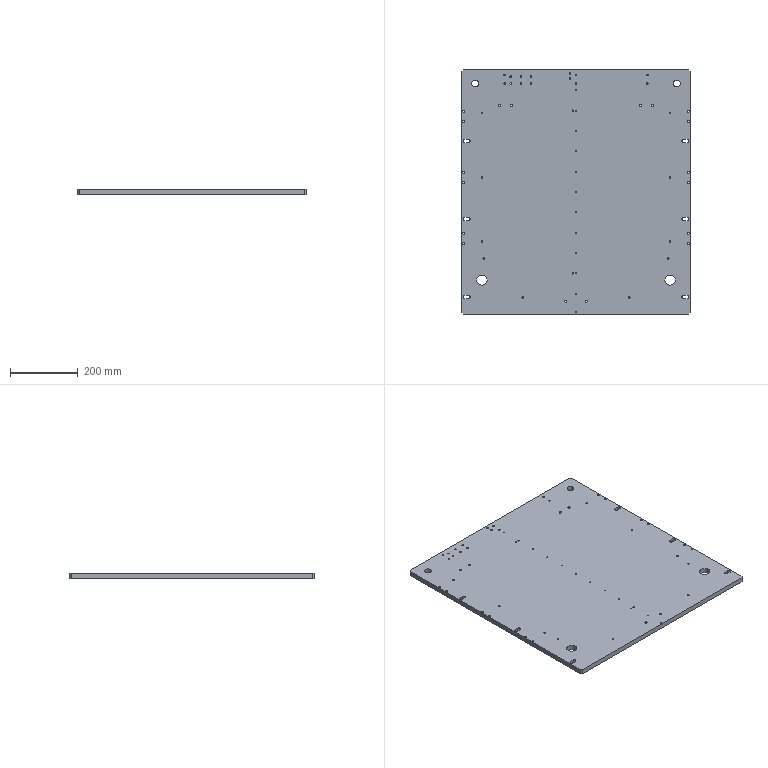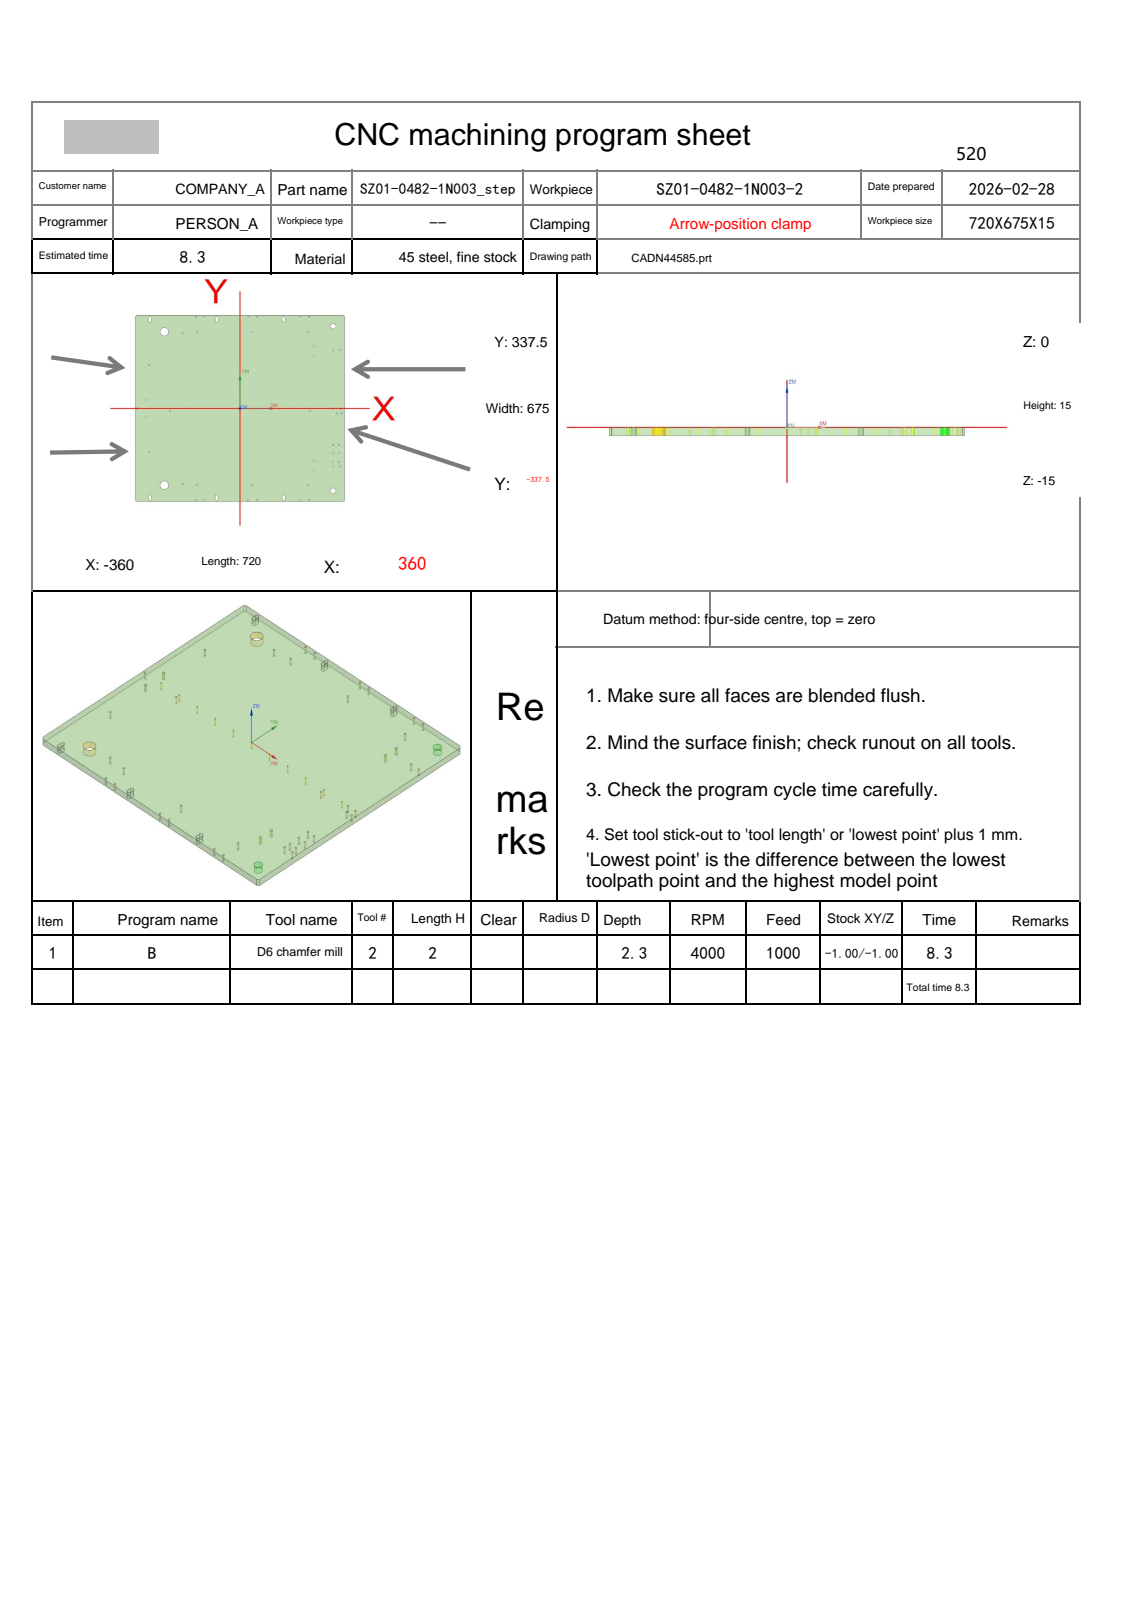NC program | NX | posted by the shop | part box 675 x 720 x 15 mm
Whole program:
%
O0001
(Machine time: 7.95 MIN)
(===Total Tool:1===)
(T2=D6 chamfer mill   D=6.   R=0.   D-  H02 Z=-2.3  )
G80 G90 G17 G49 G40
G91 G28 Z0
M01
N1 T02 M06
(D6 chamfer mill  D=6. R=0. H=02 ce=0.00 di=0.00)
G00 G90 G54 X300. Y0.0 M03 S2000
G43 H02 Z50.
M08
G98 G81 X300. Y0.0 Z-2.2 R3. F100.
X240.
X180.
X120.
X60.
X0.0
X-60.
X-120.
X-180.
X-240.
X-300.
G80
G00 Z50.
G00 G90 X240. Y-9.5 M03 S2000
Z50.
G98 G81 X240. Y-9.5 Z-2.3 R3. F100.
X-240.
G80
G00 Z50.
G00 G90 X319.306 Y-.093 M03 S4000
Z50.
Z-1.1
G01 Z-1.6 F300.
X318.5 Y-.2
G03 X320. Y-1.7 I1.5 J0.0
X321.7 Y0.0 I0.0 J1.7
X320. Y1.7 I-1.7 J0.0
X318.3 Y0.0 I0.0 J-1.7
X320. Y-1.7 I1.7 J0.0
X321.5 Y-.2 I0.0 J1.5
G01 X320.694 Y-.093
Z-1.1
G00 Z50.
X344.306
Z-1.1
G01 Z-1.6
X343.5 Y-.2
G03 X345. Y-1.7 I1.5 J0.0
X346.7 Y0.0 I0.0 J1.7
X345. Y1.7 I-1.7 J0.0
X343.3 Y0.0 I0.0 J-1.7
X345. Y-1.7 I1.7 J0.0
X346.5 Y-.2 I0.0 J1.5
G01 X345.694 Y-.093
Z-1.1
G00 Z50.
X349.306 Y-18.093
Z-1.1
G01 Z-1.6
X348.5 Y-18.2
G03 X350. Y-19.7 I1.5 J0.0
X351.7 Y-18. I0.0 J1.7
X350. Y-16.3 I-1.7 J0.0
X348.3 Y-18. I0.0 J-1.7
X350. Y-19.7 I1.7 J0.0
X351.5 Y-18.2 I0.0 J1.5
G01 X350.694 Y-18.093
Z-1.1
G00 Z50.
X333.306
Z-1.1
G01 Z-1.6
X332.5 Y-18.2
G03 X334. Y-19.7 I1.5 J0.0
X335.7 Y-18. I0.0 J1.7
X334. Y-16.3 I-1.7 J0.0
X332.3 Y-18. I0.0 J-1.7
X334. Y-19.7 I1.7 J0.0
X335.5 Y-18.2 I0.0 J1.5
G01 X334.694 Y-18.093
Z-1.1
G00 Z50.
X320.694 Y-132.407
Z-1.1
G01 Z-1.6
X321.5 Y-132.3
G03 X320. Y-130.8 I-1.5 J0.0
X318.3 Y-132.5 I0.0 J-1.7
X320. Y-134.2 I1.7 J0.0
X321.7 Y-132.5 I0.0 J1.7
X320. Y-130.8 I-1.7 J0.0
X318.5 Y-132.3 I0.0 J-1.5
G01 X319.306 Y-132.407
Z-1.1
G00 Z50.
X340.694
Z-1.1
G01 Z-1.6
X341.5 Y-132.3
G03 X340. Y-130.8 I-1.5 J0.0
X338.3 Y-132.5 I0.0 J-1.7
X340. Y-134.2 I1.7 J0.0
X341.7 Y-132.5 I0.0 J1.7
X340. Y-130.8 I-1.7 J0.0
X338.5 Y-132.3 I0.0 J-1.5
G01 X339.306 Y-132.407
Z-1.1
G00 Z50.
X340.694 Y-162.407
Z-1.1
G01 Z-1.6
X341.5 Y-162.3
G03 X340. Y-160.8 I-1.5 J0.0
X338.3 Y-162.5 I0.0 J-1.7
X340. Y-164.2 I1.7 J0.0
X341.7 Y-162.5 I0.0 J1.7
X340. Y-160.8 I-1.7 J0.0
X338.5 Y-162.3 I0.0 J-1.5
G01 X339.306 Y-162.407
Z-1.1
G00 Z50.
X320.694
Z-1.1
G01 Z-1.6
X321.5 Y-162.3
G03 X320. Y-160.8 I-1.5 J0.0
X318.3 Y-162.5 I0.0 J-1.7
X320. Y-164.2 I1.7 J0.0
X321.7 Y-162.5 I0.0 J1.7
X320. Y-160.8 I-1.7 J0.0
X318.5 Y-162.3 I0.0 J-1.5
G01 X319.306 Y-162.407
Z-1.1
G00 Z50.
X320.694 Y-192.407
Z-1.1
G01 Z-1.6
X321.5 Y-192.3
G03 X320. Y-190.8 I-1.5 J0.0
X318.3 Y-192.5 I0.0 J-1.7
X320. Y-194.2 I1.7 J0.0
X321.7 Y-192.5 I0.0 J1.7
X320. Y-190.8 I-1.7 J0.0
X318.5 Y-192.3 I0.0 J-1.5
G01 X319.306 Y-192.407
Z-1.1
G00 Z50.
X340.694
Z-1.1
G01 Z-1.6
X341.5 Y-192.3
G03 X340. Y-190.8 I-1.5 J0.0
X338.3 Y-192.5 I0.0 J-1.7
X340. Y-194.2 I1.7 J0.0
X341.7 Y-192.5 I0.0 J1.7
X340. Y-190.8 I-1.7 J0.0
X338.5 Y-192.3 I0.0 J-1.5
G01 X339.306 Y-192.407
Z-1.1
G00 Z50.
X344.306 Y-210.093
Z-1.1
G01 Z-1.6
X343.5 Y-210.2
G03 X345. Y-211.7 I1.5 J0.0
X346.7 Y-210. I0.0 J1.7
X345. Y-208.3 I-1.7 J0.0
X343.3 Y-210. I0.0 J-1.7
X345. Y-211.7 I1.7 J0.0
X346.5 Y-210.2 I0.0 J1.5
G01 X345.694 Y-210.093
Z-1.1
G00 Z50.
X319.306
Z-1.1
G01 Z-1.6
X318.5 Y-210.2
G03 X320. Y-211.7 I1.5 J0.0
X321.7 Y-210. I0.0 J1.7
X320. Y-208.3 I-1.7 J0.0
X318.3 Y-210. I0.0 J-1.7
X320. Y-211.7 I1.7 J0.0
X321.5 Y-210.2 I0.0 J1.5
G01 X320.694 Y-210.093
Z-1.1
G00 Z50.
X232.306 Y-277.093
Z-1.1
G01 Z-1.6
X231.5 Y-277.2
G03 X233. Y-278.7 I1.5 J0.0
X234.7 Y-277. I0.0 J1.7
X233. Y-275.3 I-1.7 J0.0
X231.3 Y-277. I0.0 J-1.7
X233. Y-278.7 I1.7 J0.0
X234.5 Y-277.2 I0.0 J1.5
G01 X233.694 Y-277.093
Z-1.1
G00 Z50.
X237.306 Y-331.593
Z-1.1
G01 Z-1.6
X236.5 Y-331.7
G03 X238. Y-333.2 I1.5 J0.0
X239.7 Y-331.5 I0.0 J1.7
X238. Y-329.8 I-1.7 J0.0
X236.3 Y-331.5 I0.0 J-1.7
X238. Y-333.2 I1.7 J0.0
X239.5 Y-331.7 I0.0 J1.5
G01 X238.694 Y-331.593
Z-1.1
G00 Z50.
X207.306
Z-1.1
G01 Z-1.6
X206.5 Y-331.7
G03 X208. Y-333.2 I1.5 J0.0
X209.7 Y-331.5 I0.0 J1.7
X208. Y-329.8 I-1.7 J0.0
X206.3 Y-331.5 I0.0 J-1.7
X208. Y-333.2 I1.7 J0.0
X209.5 Y-331.7 I0.0 J1.5
G01 X208.694 Y-331.593
Z-1.1
G00 Z50.
X57.306
Z-1.1
G01 Z-1.6
X56.5 Y-331.7
G03 X58. Y-333.2 I1.5 J0.0
X59.7 Y-331.5 I0.0 J1.7
X58. Y-329.8 I-1.7 J0.0
X56.3 Y-331.5 I0.0 J-1.7
X58. Y-333.2 I1.7 J0.0
X59.5 Y-331.7 I0.0 J1.5
G01 X58.694 Y-331.593
Z-1.1
G00 Z50.
X42.306 Y-277.093
Z-1.1
G01 Z-1.6
X41.5 Y-277.2
G03 X43. Y-278.7 I1.5 J0.0
X44.7 Y-277. I0.0 J1.7
X43. Y-275.3 I-1.7 J0.0
X41.3 Y-277. I0.0 J-1.7
X43. Y-278.7 I1.7 J0.0
X44.5 Y-277.2 I0.0 J1.5
G01 X43.694 Y-277.093
Z-1.1
G00 Z50.
X27.306 Y-331.593
Z-1.1
G01 Z-1.6
X26.5 Y-331.7
G03 X28. Y-333.2 I1.5 J0.0
X29.7 Y-331.5 I0.0 J1.7
X28. Y-329.8 I-1.7 J0.0
X26.3 Y-331.5 I0.0 J-1.7
X28. Y-333.2 I1.7 J0.0
X29.5 Y-331.7 I0.0 J1.5
G01 X28.694 Y-331.593
Z-1.1
G00 Z50.
X-122.694
Z-1.1
G01 Z-1.6
X-123.5 Y-331.7
G03 X-122. Y-333.2 I1.5 J0.0
X-120.3 Y-331.5 I0.0 J1.7
X-122. Y-329.8 I-1.7 J0.0
X-123.7 Y-331.5 I0.0 J-1.7
X-122. Y-333.2 I1.7 J0.0
X-120.5 Y-331.7 I0.0 J1.5
G01 X-121.306 Y-331.593
Z-1.1
G00 Z50.
X-152.694
Z-1.1
G01 Z-1.6
X-153.5 Y-331.7
G03 X-152. Y-333.2 I1.5 J0.0
X-150.3 Y-331.5 I0.0 J1.7
X-152. Y-329.8 I-1.7 J0.0
X-153.7 Y-331.5 I0.0 J-1.7
X-152. Y-333.2 I1.7 J0.0
X-150.5 Y-331.7 I0.0 J1.5
G01 X-151.306 Y-331.593
Z-1.1
G00 Z50.
X-147.694 Y-277.093
Z-1.1
G01 Z-1.6
X-148.5 Y-277.2
G03 X-147. Y-278.7 I1.5 J0.0
X-145.3 Y-277. I0.0 J1.7
X-147. Y-275.3 I-1.7 J0.0
X-148.7 Y-277. I0.0 J-1.7
X-147. Y-278.7 I1.7 J0.0
X-145.5 Y-277.2 I0.0 J1.5
G01 X-146.306 Y-277.093
Z-1.1
G00 Z50.
X-197.694 Y-272.024
Z-1.1
G01 Z-1.6
X-198.5 Y-272.132
G03 X-197. Y-273.632 I1.5 J0.0
X-195.3 Y-271.932 I0.0 J1.7
X-197. Y-270.232 I-1.7 J0.0
X-198.7 Y-271.932 I0.0 J-1.7
X-197. Y-273.632 I1.7 J0.0
X-195.5 Y-272.132 I0.0 J1.5
G01 X-196.306 Y-272.024
Z-1.1
G00 Z50.
X-312.626 Y-157.093
Z-1.1
G01 Z-1.6
X-313.432 Y-157.2
G03 X-311.932 Y-158.7 I1.5 J0.0
X-310.232 Y-157. I0.0 J1.7
X-311.932 Y-155.3 I-1.7 J0.0
X-313.632 Y-157. I0.0 J-1.7
X-311.932 Y-158.7 I1.7 J0.0
X-310.432 Y-157.2 I0.0 J1.5
G01 X-311.238 Y-157.093
Z-1.1
G00 Z50.
X-354.694 Y-.093
Z-1.1
G01 Z-1.6
X-355.5 Y-.2
G03 X-354. Y-1.7 I1.5 J0.0
X-352.3 Y0.0 I0.0 J1.7
X-354. Y1.7 I-1.7 J0.0
X-355.7 Y0.0 I0.0 J-1.7
X-354. Y-1.7 I1.7 J0.0
X-352.5 Y-.2 I0.0 J1.5
G01 X-353.306 Y-.093
Z-1.1
G00 Z50.
X-312.626 Y156.907
Z-1.1
G01 Z-1.6
X-313.432 Y156.8
G03 X-311.932 Y155.3 I1.5 J0.0
X-310.232 Y157. I0.0 J1.7
X-311.932 Y158.7 I-1.7 J0.0
X-313.632 Y157. I0.0 J-1.7
X-311.932 Y155.3 I1.7 J0.0
X-310.432 Y156.8 I0.0 J1.5
G01 X-311.238 Y156.907
Z-1.1
G00 Z50.
X-197.694 Y271.839
Z-1.1
G01 Z-1.6
X-198.5 Y271.732
G03 X-197. Y270.232 I1.5 J0.0
X-195.3 Y271.932 I0.0 J1.7
X-197. Y273.632 I-1.7 J0.0
X-198.7 Y271.932 I0.0 J-1.7
X-197. Y270.232 I1.7 J0.0
X-195.5 Y271.732 I0.0 J1.5
G01 X-196.306 Y271.839
Z-1.1
G00 Z50.
X-147.694 Y276.907
Z-1.1
G01 Z-1.6
X-148.5 Y276.8
G03 X-147. Y275.3 I1.5 J0.0
X-145.3 Y277. I0.0 J1.7
X-147. Y278.7 I-1.7 J0.0
X-148.7 Y277. I0.0 J-1.7
X-147. Y275.3 I1.7 J0.0
X-145.5 Y276.8 I0.0 J1.5
G01 X-146.306 Y276.907
Z-1.1
G00 Z50.
X-152.694 Y331.407
Z-1.1
G01 Z-1.6
X-153.5 Y331.3
G03 X-152. Y329.8 I1.5 J0.0
X-150.3 Y331.5 I0.0 J1.7
X-152. Y333.2 I-1.7 J0.0
X-153.7 Y331.5 I0.0 J-1.7
X-152. Y329.8 I1.7 J0.0
X-150.5 Y331.3 I0.0 J1.5
G01 X-151.306 Y331.407
Z-1.1
G00 Z50.
X-122.694
Z-1.1
G01 Z-1.6
X-123.5 Y331.3
G03 X-122. Y329.8 I1.5 J0.0
X-120.3 Y331.5 I0.0 J1.7
X-122. Y333.2 I-1.7 J0.0
X-123.7 Y331.5 I0.0 J-1.7
X-122. Y329.8 I1.7 J0.0
X-120.5 Y331.3 I0.0 J1.5
G01 X-121.306 Y331.407
Z-1.1
G00 Z50.
X27.306
Z-1.1
G01 Z-1.6
X26.5 Y331.3
G03 X28. Y329.8 I1.5 J0.0
X29.7 Y331.5 I0.0 J1.7
X28. Y333.2 I-1.7 J0.0
X26.3 Y331.5 I0.0 J-1.7
X28. Y329.8 I1.7 J0.0
X29.5 Y331.3 I0.0 J1.5
G01 X28.694 Y331.407
Z-1.1
G00 Z50.
X42.306 Y276.907
Z-1.1
G01 Z-1.6
X41.5 Y276.8
G03 X43. Y275.3 I1.5 J0.0
X44.7 Y277. I0.0 J1.7
X43. Y278.7 I-1.7 J0.0
X41.3 Y277. I0.0 J-1.7
X43. Y275.3 I1.7 J0.0
X44.5 Y276.8 I0.0 J1.5
G01 X43.694 Y276.907
Z-1.1
G00 Z50.
X57.306 Y331.407
Z-1.1
G01 Z-1.6
X56.5 Y331.3
G03 X58. Y329.8 I1.5 J0.0
X59.7 Y331.5 I0.0 J1.7
X58. Y333.2 I-1.7 J0.0
X56.3 Y331.5 I0.0 J-1.7
X58. Y329.8 I1.7 J0.0
X59.5 Y331.3 I0.0 J1.5
G01 X58.694 Y331.407
Z-1.1
G00 Z50.
X207.306
Z-1.1
G01 Z-1.6
X206.5 Y331.3
G03 X208. Y329.8 I1.5 J0.0
X209.7 Y331.5 I0.0 J1.7
X208. Y333.2 I-1.7 J0.0
X206.3 Y331.5 I0.0 J-1.7
X208. Y329.8 I1.7 J0.0
X209.5 Y331.3 I0.0 J1.5
G01 X208.694 Y331.407
Z-1.1
G00 Z50.
X237.306
Z-1.1
G01 Z-1.6
X236.5 Y331.3
G03 X238. Y329.8 I1.5 J0.0
X239.7 Y331.5 I0.0 J1.7
X238. Y333.2 I-1.7 J0.0
X236.3 Y331.5 I0.0 J-1.7
X238. Y329.8 I1.7 J0.0
X239.5 Y331.3 I0.0 J1.5
G01 X238.694 Y331.407
Z-1.1
G00 Z50.
X232.306 Y276.907
Z-1.1
G01 Z-1.6
X231.5 Y276.8
G03 X233. Y275.3 I1.5 J0.0
X234.7 Y277. I0.0 J1.7
X233. Y278.7 I-1.7 J0.0
X231.3 Y277. I0.0 J-1.7
X233. Y275.3 I1.7 J0.0
X234.5 Y276.8 I0.0 J1.5
G01 X233.694 Y276.907
Z-1.1
G00 Z50.
X319.306 Y209.907
Z-1.1
G01 Z-1.6
X318.5 Y209.8
G03 X320. Y208.3 I1.5 J0.0
X321.7 Y210. I0.0 J1.7
X320. Y211.7 I-1.7 J0.0
X318.3 Y210. I0.0 J-1.7
X320. Y208.3 I1.7 J0.0
X321.5 Y209.8 I0.0 J1.5
G01 X320.694 Y209.907
Z-1.1
G00 Z50.
X344.306
Z-1.1
G01 Z-1.6
X343.5 Y209.8
G03 X345. Y208.3 I1.5 J0.0
X346.7 Y210. I0.0 J1.7
X345. Y211.7 I-1.7 J0.0
X343.3 Y210. I0.0 J-1.7
X345. Y208.3 I1.7 J0.0
X346.5 Y209.8 I0.0 J1.5
G01 X345.694 Y209.907
Z-1.1
G00 Z50.
G00 G90 X-323.5 Y-30.995 M03 S4000
Z50.
Z-1.1
G01 Z-1.6 F300.
Y-31.3
G03 X-322. Y-32.8 I1.5 J0.0
X-319.2 Y-30. I0.0 J2.8
X-322. Y-27.2 I-2.8 J0.0
X-324.8 Y-30. I0.0 J-2.8
X-322. Y-32.8 I2.8 J0.0
X-320.5 Y-31.3 I0.0 J1.5
G01 Y-30.995
Z-1.1
G00 Z50.
X-323.5 Y29.005
Z-1.1
G01 Z-1.6
Y28.7
G03 X-322. Y27.2 I1.5 J0.0
X-319.2 Y30. I0.0 J2.8
X-322. Y32.8 I-2.8 J0.0
X-324.8 Y30. I0.0 J-2.8
X-322. Y27.2 I2.8 J0.0
X-320.5 Y28.7 I0.0 J1.5
G01 Y29.005
Z-1.1
G00 Z50.
X253.5 Y224.505
Z-1.1
G01 Z-1.6
Y224.2
G03 X255. Y222.7 I1.5 J0.0
X257.8 Y225.5 I0.0 J2.8
X255. Y228.3 I-2.8 J0.0
X252.2 Y225.5 I0.0 J-2.8
X255. Y222.7 I2.8 J0.0
X256.5 Y224.2 I0.0 J1.5
G01 Y224.505
Z-1.1
G00 Z50.
X253.5 Y188.505
Z-1.1
G01 Z-1.6
Y188.2
G03 X255. Y186.7 I1.5 J0.0
X257.8 Y189.5 I0.0 J2.8
X255. Y192.3 I-2.8 J0.0
X252.2 Y189.5 I0.0 J-2.8
X255. Y186.7 I2.8 J0.0
X256.5 Y188.2 I0.0 J1.5
G01 Y188.505
Z-1.1
G00 Z50.
X253.5 Y-190.495
Z-1.1
G01 Z-1.6
Y-190.8
G03 X255. Y-192.3 I1.5 J0.0
X257.8 Y-189.5 I0.0 J2.8
X255. Y-186.7 I-2.8 J0.0
X252.2 Y-189.5 I0.0 J-2.8
X255. Y-192.3 I2.8 J0.0
X256.5 Y-190.8 I0.0 J1.5
G01 Y-190.495
Z-1.1
G00 Z50.
X253.5 Y-226.495
Z-1.1
G01 Z-1.6
Y-226.8
G03 X255. Y-228.3 I1.5 J0.0
X257.8 Y-225.5 I0.0 J2.8
X255. Y-222.7 I-2.8 J0.0
X252.2 Y-225.5 I0.0 J-2.8
X255. Y-228.3 I2.8 J0.0
X256.5 Y-226.8 I0.0 J1.5
G01 Y-226.495
Z-1.1
G00 Z50.
G00 G90 X-361.275 Y332.147 M03 S3500
Z50.
Z.124
G01 Z-1.2 F1000.
G03 X-361.04 Y332.404 I-1.351 J1.475
G01 X-361.004 Y332.446
X-361. Y332.5
X-360.966 Y332.759
X-360.866 Y333.
X-360.707 Y333.207
X-355.707 Y338.207
X-355.5 Y338.366
X-355.259 Y338.466
X-355. Y338.5
X355.
X355.259 Y338.466
X355.5 Y338.366
X355.707 Y338.207
X360.707 Y333.207
X360.744 Y333.167
X360.797 Y333.155
G03 X361.14 Y333.095 I.518 J1.932
G01 Z.113
G00 Z50.
X361.275 Y-332.147
Z.124
G01 Z-1.2
G03 X361.04 Y-332.404 I1.351 J-1.475
G01 X361.004 Y-332.446
X361. Y-332.5
X360.966 Y-332.759
X360.866 Y-333.
X360.707 Y-333.207
X355.707 Y-338.207
X355.5 Y-338.366
X355.259 Y-338.466
X355. Y-338.5
X-355.
X-355.259 Y-338.466
X-355.5 Y-338.366
X-355.707 Y-338.207
X-360.707 Y-333.207
X-360.744 Y-333.167
X-360.797 Y-333.155
G03 X-361.14 Y-333.095 I-.518 J-1.932
G01 Z.113
G00 Z50.
X319.605 Y-306.29
Z.199
G01 Z-1.2
G03 X319.899 Y-306.478 I1.218 J1.587
G01 X319.946 Y-306.505
X320. Y-306.5
G03 X329. Y-297.5 I0.0 J9.
X320. Y-288.5 I-9. J0.0
X311. Y-297.5 I0.0 J-9.
X320. Y-306.5 I9. J0.0
G01 X320.054 Y-306.505
X320.101 Y-306.478
G03 X320.395 Y-306.29 I-.923 J1.774
G01 Z.199
G00 Z50.
X344.593 Y-211.315
Z.284
G01 Z-1.2
G03 X344.898 Y-211.484 I1.118 J1.658
G01 X344.946 Y-211.509
X345. Y-211.5
G03 X346.5 Y-210. I0.0 J1.5
X345. Y-208.5 I-1.5 J0.0
X343.5 Y-210. I0.0 J-1.5
X345. Y-211.5 I1.5 J0.0
G01 X345.054 Y-211.509
X345.102 Y-211.484
G03 X345.407 Y-211.315 I-.813 J1.827
G01 Z.284
G00 Z50.
X340.407 Y-191.185
Z.284
G01 Z-1.2
G03 X340.102 Y-191.016 I-1.118 J-1.658
G01 X340.054 Y-190.991
X340. Y-191.
G03 X338.5 Y-192.5 I0.0 J-1.5
X340. Y-194. I1.5 J0.0
X341.5 Y-192.5 I0.0 J1.5
X340. Y-191. I-1.5 J0.0
G01 X339.946 Y-190.991
X339.898 Y-191.016
G03 X339.593 Y-191.185 I.813 J-1.827
G01 Z.284
G00 Z50.
X340.407 Y-161.185
Z.284
G01 Z-1.2
G03 X340.102 Y-161.016 I-1.118 J-1.658
G01 X340.054 Y-160.991
X340. Y-161.
G03 X338.5 Y-162.5 I0.0 J-1.5
X340. Y-164. I1.5 J0.0
X341.5 Y-162.5 I0.0 J1.5
X340. Y-161. I-1.5 J0.0
G01 X339.946 Y-160.991
X339.898 Y-161.016
G03 X339.593 Y-161.185 I.813 J-1.827
G01 Z.284
G00 Z50.
X340.407 Y-131.185
Z.284
G01 Z-1.2
G03 X340.102 Y-131.016 I-1.118 J-1.658
G01 X340.054 Y-130.991
X340. Y-131.
G03 X338.5 Y-132.5 I0.0 J-1.5
X340. Y-134. I1.5 J0.0
X341.5 Y-132.5 I0.0 J1.5
X340. Y-131. I-1.5 J0.0
G01 X339.946 Y-130.991
X339.898 Y-131.016
G03 X339.593 Y-131.185 I.813 J-1.827
G01 Z.284
G00 Z50.
X320.407
Z.284
G01 Z-1.2
G03 X320.102 Y-131.016 I-1.118 J-1.658
G01 X320.054 Y-130.991
X320. Y-131.
G03 X318.5 Y-132.5 I0.0 J-1.5
X320. Y-134. I1.5 J0.0
X321.5 Y-132.5 I0.0 J1.5
X320. Y-131. I-1.5 J0.0
G01 X319.946 Y-130.991
X319.898 Y-131.016
G03 X319.593 Y-131.185 I.813 J-1.827
G01 Z.284
G00 Z50.
X320.407 Y-161.185
Z.284
G01 Z-1.2
G03 X320.102 Y-161.016 I-1.118 J-1.658
G01 X320.054 Y-160.991
X320. Y-161.
G03 X318.5 Y-162.5 I0.0 J-1.5
X320. Y-164. I1.5 J0.0
X321.5 Y-162.5 I0.0 J1.5
X320. Y-161. I-1.5 J0.0
G01 X319.946 Y-160.991
X319.898 Y-161.016
G03 X319.593 Y-161.185 I.813 J-1.827
G01 Z.284
G00 Z50.
X320.407 Y-191.185
Z.284
G01 Z-1.2
G03 X320.102 Y-191.016 I-1.118 J-1.658
G01 X320.054 Y-190.991
X320. Y-191.
G03 X318.5 Y-192.5 I0.0 J-1.5
X320. Y-194. I1.5 J0.0
X321.5 Y-192.5 I0.0 J1.5
X320. Y-191. I-1.5 J0.0
G01 X319.946 Y-190.991
X319.898 Y-191.016
G03 X319.593 Y-191.185 I.813 J-1.827
G01 Z.284
G00 Z50.
Y-211.315
Z.284
G01 Z-1.2
G03 X319.898 Y-211.484 I1.118 J1.658
G01 X319.946 Y-211.509
X320. Y-211.5
G03 X321.5 Y-210. I0.0 J1.5
X320. Y-208.5 I-1.5 J0.0
X318.5 Y-210. I0.0 J-1.5
X320. Y-211.5 I1.5 J0.0
G01 X320.054 Y-211.509
X320.102 Y-211.484
G03 X320.407 Y-211.315 I-.813 J1.827
G01 Z.284
G00 Z50.
X254.596 Y-191.708
Z.252
G01 Z-1.2
G03 X254.898 Y-191.882 I1.147 J1.638
G01 X254.946 Y-191.908
X255. Y-191.9
G03 X257.4 Y-189.5 I0.0 J2.4
X255. Y-187.1 I-2.4 J0.0
X252.6 Y-189.5 I0.0 J-2.4
X255. Y-191.9 I2.4 J0.0
G01 X255.054 Y-191.908
X255.102 Y-191.882
G03 X255.404 Y-191.708 I-.845 J1.813
G01 Z.252
G00 Z50.
X254.596 Y-227.708
Z.252
G01 Z-1.2
G03 X254.898 Y-227.882 I1.147 J1.638
G01 X254.946 Y-227.908
X255. Y-227.9
G03 X257.4 Y-225.5 I0.0 J2.4
X255. Y-223.1 I-2.4 J0.0
X252.6 Y-225.5 I0.0 J-2.4
X255. Y-227.9 I2.4 J0.0
G01 X255.054 Y-227.908
X255.102 Y-227.882
G03 X255.404 Y-227.708 I-.845 J1.813
G01 Z.252
G00 Z50.
X232.593 Y-278.315
Z.284
G01 Z-1.2
G03 X232.898 Y-278.484 I1.118 J1.658
G01 X232.946 Y-278.509
X233. Y-278.5
G03 X234.5 Y-277. I0.0 J1.5
X233. Y-275.5 I-1.5 J0.0
X231.5 Y-277. I0.0 J-1.5
X233. Y-278.5 I1.5 J0.0
G01 X233.054 Y-278.509
X233.102 Y-278.484
G03 X233.407 Y-278.315 I-.813 J1.827
G01 Z.284
G00 Z50.
X237.593 Y-332.815
Z.284
G01 Z-1.2
G03 X237.898 Y-332.984 I1.118 J1.658
G01 X237.946 Y-333.009
X238. Y-333.
G03 X239.5 Y-331.5 I0.0 J1.5
X238. Y-330. I-1.5 J0.0
X236.5 Y-331.5 I0.0 J-1.5
X238. Y-333. I1.5 J0.0
G01 X238.054 Y-333.009
X238.102 Y-332.984
G03 X238.407 Y-332.815 I-.813 J1.827
G01 Z.284
G00 Z50.
X207.593
Z.284
G01 Z-1.2
G03 X207.898 Y-332.984 I1.118 J1.658
G01 X207.946 Y-333.009
X208. Y-333.
G03 X209.5 Y-331.5 I0.0 J1.5
X208. Y-330. I-1.5 J0.0
X206.5 Y-331.5 I0.0 J-1.5
X208. Y-333. I1.5 J0.0
G01 X208.054 Y-333.009
X208.102 Y-332.984
G03 X208.407 Y-332.815 I-.813 J1.827
G01 Z.284
G00 Z50.
X153.773 Y-322.886
Z.172
G01 Z-1.2
G03 X153.973 Y-322.6 I-1.532 J1.286
G01 X154.003 Y-322.554
X154. Y-322.5
Y-317.5
G03 X150. Y-313.5 I-4. J0.0
X146. Y-317.5 I0.0 J-4.
G01 Y-327.5
G03 X150. Y-331.5 I4. J0.0
X154. Y-327.5 I0.0 J4.
G01 Y-322.5
X154.003 Y-322.446
X153.973 Y-322.4
G03 X153.773 Y-322.114 I-1.732 J-1.
G01 Z.172
G00 Z50.
X57.593 Y-332.815
Z.284
G01 Z-1.2
G03 X57.898 Y-332.984 I1.118 J1.658
G01 X57.946 Y-333.009
X58. Y-333.
G03 X59.5 Y-331.5 I0.0 J1.5
X58. Y-330. I-1.5 J0.0
X56.5 Y-331.5 I0.0 J-1.5
X58. Y-333. I1.5 J0.0
G01 X58.054 Y-333.009
X58.102 Y-332.984
G03 X58.407 Y-332.815 I-.813 J1.827
G01 Z.284
G00 Z50.
X27.593
Z.284
G01 Z-1.2
G03 X27.898 Y-332.984 I1.118 J1.658
G01 X27.946 Y-333.009
X28. Y-333.
G03 X29.5 Y-331.5 I0.0 J1.5
X28. Y-330. I-1.5 J0.0
X26.5 Y-331.5 I0.0 J-1.5
X28. Y-333. I1.5 J0.0
G01 X28.054 Y-333.009
X28.102 Y-332.984
G03 X28.407 Y-332.815 I-.813 J1.827
G01 Z.284
G00 Z50.
X42.593 Y-278.315
Z.284
G01 Z-1.2
G03 X42.898 Y-278.484 I1.118 J1.658
G01 X42.946 Y-278.509
X43. Y-278.5
G03 X44.5 Y-277. I0.0 J1.5
X43. Y-275.5 I-1.5 J0.0
X41.5 Y-277. I0.0 J-1.5
X43. Y-278.5 I1.5 J0.0
G01 X43.054 Y-278.509
X43.102 Y-278.484
G03 X43.407 Y-278.315 I-.813 J1.827
G01 Z.284
G00 Z50.
X-76.227 Y-322.886
Z.172
G01 Z-1.2
G03 X-76.027 Y-322.6 I-1.532 J1.286
G01 X-75.997 Y-322.554
X-76. Y-322.5
Y-317.5
G03 X-80. Y-313.5 I-4. J0.0
X-84. Y-317.5 I0.0 J-4.
G01 Y-327.5
G03 X-80. Y-331.5 I4. J0.0
X-76. Y-327.5 I0.0 J4.
G01 Y-322.5
X-75.997 Y-322.446
X-76.027 Y-322.4
G03 X-76.227 Y-322.114 I-1.732 J-1.
G01 Z.172
G00 Z50.
X-122.407 Y-332.815
Z.284
G01 Z-1.2
G03 X-122.102 Y-332.984 I1.118 J1.658
G01 X-122.054 Y-333.009
X-122. Y-333.
G03 X-120.5 Y-331.5 I0.0 J1.5
X-122. Y-330. I-1.5 J0.0
X-123.5 Y-331.5 I0.0 J-1.5
X-122. Y-333. I1.5 J0.0
G01 X-121.946 Y-333.009
X-121.898 Y-332.984
G03 X-121.593 Y-332.815 I-.813 J1.827
G01 Z.284
G00 Z50.
X-152.407
Z.284
G01 Z-1.2
G03 X-152.102 Y-332.984 I1.118 J1.658
G01 X-152.054 Y-333.009
X-152. Y-333.
G03 X-150.5 Y-331.5 I0.0 J1.5
X-152. Y-330. I-1.5 J0.0
X-153.5 Y-331.5 I0.0 J-1.5
X-152. Y-333. I1.5 J0.0
G01 X-151.946 Y-333.009
X-151.898 Y-332.984
G03 X-151.593 Y-332.815 I-.813 J1.827
G01 Z.284
G00 Z50.
X-147.407 Y-278.315
Z.284
G01 Z-1.2
G03 X-147.102 Y-278.484 I1.118 J1.658
G01 X-147.054 Y-278.509
X-147. Y-278.5
G03 X-145.5 Y-277. I0.0 J1.5
X-147. Y-275.5 I-1.5 J0.0
X-148.5 Y-277. I0.0 J-1.5
X-147. Y-278.5 I1.5 J0.0
G01 X-146.946 Y-278.509
X-146.898 Y-278.484
G03 X-146.593 Y-278.315 I-.813 J1.827
G01 Z.284
G00 Z50.
X-197.407 Y-273.247
Z.284
G01 Z-1.2
G03 X-197.102 Y-273.416 I1.118 J1.658
G01 X-197.054 Y-273.44
X-197. Y-273.432
G03 X-195.5 Y-271.932 I0.0 J1.5
X-197. Y-270.432 I-1.5 J0.0
X-198.5 Y-271.932 I0.0 J-1.5
X-197. Y-273.432 I1.5 J0.0
G01 X-196.946 Y-273.44
X-196.898 Y-273.416
G03 X-196.593 Y-273.247 I-.813 J1.827
G01 Z.284
G00 Z50.
X-260.394 Y-291.288
Z.196
G01 Z-1.2
G03 X-260.101 Y-291.477 I1.227 J1.579
G01 X-260.054 Y-291.505
X-260. Y-291.5
G03 X-246. Y-277.5 I0.0 J14.
X-260. Y-263.5 I-14. J0.0
X-274. Y-277.5 I0.0 J-14.
X-260. Y-291.5 I14. J0.0
G01 X-259.946 Y-291.505
X-259.899 Y-291.477
G03 X-259.606 Y-291.288 I-.935 J1.768
G01 Z.196
G00 Z50.
X-306.227 Y-322.886
Z.172
G01 Z-1.2
G03 X-306.027 Y-322.6 I-1.532 J1.286
G01 X-305.997 Y-322.554
X-306. Y-322.5
Y-317.5
G03 X-310. Y-313.5 I-4. J0.0
X-314. Y-317.5 I0.0 J-4.
G01 Y-327.5
G03 X-310. Y-331.5 I4. J0.0
X-306. Y-327.5 I0.0 J4.
G01 Y-322.5
X-305.997 Y-322.446
X-306.027 Y-322.4
G03 X-306.227 Y-322.114 I-1.732 J-1.
G01 Z.172
G00 Z50.
X-312.339 Y-158.315
Z.284
G01 Z-1.2
G03 X-312.034 Y-158.484 I1.118 J1.658
G01 X-311.986 Y-158.509
X-311.932 Y-158.5
G03 X-310.432 Y-157. I0.0 J1.5
X-311.932 Y-155.5 I-1.5 J0.0
X-313.432 Y-157. I0.0 J-1.5
X-311.932 Y-158.5 I1.5 J0.0
G01 X-311.878 Y-158.509
X-311.83 Y-158.484
G03 X-311.525 Y-158.315 I-.813 J1.827
G01 Z.284
G00 Z50.
X-322.404 Y-32.208
Z.252
G01 Z-1.2
G03 X-322.102 Y-32.382 I1.147 J1.638
G01 X-322.054 Y-32.408
X-322. Y-32.4
G03 X-319.6 Y-30. I0.0 J2.4
X-322. Y-27.6 I-2.4 J0.0
X-324.4 Y-30. I0.0 J-2.4
X-322. Y-32.4 I2.4 J0.0
G01 X-321.946 Y-32.408
X-321.898 Y-32.382
G03 X-321.596 Y-32.208 I-.845 J1.813
G01 Z.252
G00 Z50.
X-354.407 Y-1.315
Z.284
G01 Z-1.2
G03 X-354.102 Y-1.484 I1.118 J1.658
G01 X-354.054 Y-1.509
X-354. Y-1.5
G03 X-352.5 Y0.0 I0.0 J1.5
X-354. Y1.5 I-1.5 J0.0
X-355.5 Y0.0 I0.0 J-1.5
X-354. Y-1.5 I1.5 J0.0
G01 X-353.946 Y-1.509
X-353.898 Y-1.484
G03 X-353.593 Y-1.315 I-.813 J1.827
G01 Z.284
G00 Z50.
X-322.404 Y27.792
Z.252
G01 Z-1.2
G03 X-322.102 Y27.618 I1.147 J1.638
G01 X-322.054 Y27.592
X-322. Y27.6
G03 X-319.6 Y30. I0.0 J2.4
X-322. Y32.4 I-2.4 J0.0
X-324.4 Y30. I0.0 J-2.4
X-322. Y27.6 I2.4 J0.0
G01 X-321.946 Y27.592
X-321.898 Y27.618
G03 X-321.596 Y27.792 I-.845 J1.813
G01 Z.252
G00 Z50.
X-300.419 Y-.494
Z.405
G01 Z-1.2
G03 X-300.103 Y-.641 I1. J1.732
G01 X-300.053 Y-.662
X-300. Y-.65
G03 X-299.35 Y0.0 I0.0 J.65
X-300. Y.65 I-.65 J0.0
X-300.65 Y0.0 I0.0 J-.65
X-300. Y-.65 I.65 J0.0
G01 X-299.947 Y-.662
X-299.897 Y-.641
G03 X-299.581 Y-.494 I-.684 J1.879
G01 Z.405
G00 Z50.
X-240.412 Y-10.326
Z.33
G01 Z-1.2
G03 X-240.103 Y-10.486 I1.075 J1.687
G01 X-240.054 Y-10.51
X-240. Y-10.5
G03 X-239. Y-9.5 I0.0 J1.
X-240. Y-8.5 I-1. J0.0
X-241. Y-9.5 I0.0 J-1.
X-240. Y-10.5 I1. J0.0
G01 X-239.946 Y-10.51
X-239.897 Y-10.486
G03 X-239.588 Y-10.326 I-.765 J1.848
G01 Z.33
G00 Z2.55
X-240.419 Y-.494
Z.405
G01 Z-1.2
G03 X-240.103 Y-.641 I1. J1.732
G01 X-240.053 Y-.662
X-240. Y-.65
G03 X-239.35 Y0.0 I0.0 J.65
X-240. Y.65 I-.65 J0.0
X-240.65 Y0.0 I0.0 J-.65
X-240. Y-.65 I.65 J0.0
G01 X-239.947 Y-.662
X-239.897 Y-.641
G03 X-239.581 Y-.494 I-.684 J1.879
G01 Z.405
G00 Z50.
X-180.419
Z.405
G01 Z-1.2
G03 X-180.103 Y-.641 I1. J1.732
G01 X-180.053 Y-.662
X-180. Y-.65
G03 X-179.35 Y0.0 I0.0 J.65
X-180. Y.65 I-.65 J0.0
X-180.65 Y0.0 I0.0 J-.65
X-180. Y-.65 I.65 J0.0
G01 X-179.947 Y-.662
X-179.897 Y-.641
G03 X-179.581 Y-.494 I-.684 J1.879
G01 Z.405
G00 Z50.
X-120.419
Z.405
G01 Z-1.2
G03 X-120.103 Y-.641 I1. J1.732
G01 X-120.053 Y-.662
X-120. Y-.65
G03 X-119.35 Y0.0 I0.0 J.65
X-120. Y.65 I-.65 J0.0
X-120.65 Y0.0 I0.0 J-.65
X-120. Y-.65 I.65 J0.0
G01 X-119.947 Y-.662
X-119.897 Y-.641
G03 X-119.581 Y-.494 I-.684 J1.879
G01 Z.405
G00 Z50.
X-60.419
Z.405
G01 Z-1.2
G03 X-60.103 Y-.641 I1. J1.732
G01 X-60.053 Y-.662
X-60. Y-.65
G03 X-59.35 Y0.0 I0.0 J.65
X-60. Y.65 I-.65 J0.0
X-60.65 Y0.0 I0.0 J-.65
X-60. Y-.65 I.65 J0.0
G01 X-59.947 Y-.662
X-59.897 Y-.641
G03 X-59.581 Y-.494 I-.684 J1.879
G01 Z.405
G00 Z50.
X-.419
Z.405
G01 Z-1.2
G03 X-.103 Y-.641 I1. J1.732
G01 X-.053 Y-.662
X0.0 Y-.65
G03 X.65 Y0.0 I0.0 J.65
X0.0 Y.65 I-.65 J0.0
X-.65 Y0.0 I0.0 J-.65
X0.0 Y-.65 I.65 J0.0
G01 X.053 Y-.662
X.103 Y-.641
G03 X.419 Y-.494 I-.684 J1.879
G01 Z.405
G00 Z50.
X59.581
Z.405
G01 Z-1.2
G03 X59.897 Y-.641 I1. J1.732
G01 X59.947 Y-.662
X60. Y-.65
G03 X60.65 Y0.0 I0.0 J.65
X60. Y.65 I-.65 J0.0
X59.35 Y0.0 I0.0 J-.65
X60. Y-.65 I.65 J0.0
G01 X60.053 Y-.662
X60.103 Y-.641
G03 X60.419 Y-.494 I-.684 J1.879
G01 Z.405
G00 Z50.
X119.581
Z.405
G01 Z-1.2
G03 X119.897 Y-.641 I1. J1.732
G01 X119.947 Y-.662
X120. Y-.65
G03 X120.65 Y0.0 I0.0 J.65
X120. Y.65 I-.65 J0.0
X119.35 Y0.0 I0.0 J-.65
X120. Y-.65 I.65 J0.0
G01 X120.053 Y-.662
X120.103 Y-.641
G03 X120.419 Y-.494 I-.684 J1.879
G01 Z.405
G00 Z50.
X179.581
Z.405
G01 Z-1.2
G03 X179.897 Y-.641 I1. J1.732
G01 X179.947 Y-.662
X180. Y-.65
G03 X180.65 Y0.0 I0.0 J.65
X180. Y.65 I-.65 J0.0
X179.35 Y0.0 I0.0 J-.65
X180. Y-.65 I.65 J0.0
G01 X180.053 Y-.662
X180.103 Y-.641
G03 X180.419 Y-.494 I-.684 J1.879
G01 Z.405
G00 Z50.
X239.588 Y-10.326
Z.33
G01 Z-1.2
G03 X239.897 Y-10.486 I1.075 J1.687
G01 X239.946 Y-10.51
X240. Y-10.5
G03 X241. Y-9.5 I0.0 J1.
X240. Y-8.5 I-1. J0.0
X239. Y-9.5 I0.0 J-1.
X240. Y-10.5 I1. J0.0
G01 X240.054 Y-10.51
X240.103 Y-10.486
G03 X240.412 Y-10.326 I-.765 J1.848
G01 Z.33
G00 Z2.55
X239.581 Y-.494
Z.405
G01 Z-1.2
G03 X239.897 Y-.641 I1. J1.732
G01 X239.947 Y-.662
X240. Y-.65
G03 X240.65 Y0.0 I0.0 J.65
X240. Y.65 I-.65 J0.0
X239.35 Y0.0 I0.0 J-.65
X240. Y-.65 I.65 J0.0
G01 X240.053 Y-.662
X240.103 Y-.641
G03 X240.419 Y-.494 I-.684 J1.879
G01 Z.405
G00 Z50.
X299.581
Z.405
G01 Z-1.2
G03 X299.897 Y-.641 I1. J1.732
G01 X299.947 Y-.662
X300. Y-.65
G03 X300.65 Y0.0 I0.0 J.65
X300. Y.65 I-.65 J0.0
X299.35 Y0.0 I0.0 J-.65
X300. Y-.65 I.65 J0.0
G01 X300.053 Y-.662
X300.103 Y-.641
G03 X300.419 Y-.494 I-.684 J1.879
G01 Z.405
G00 Z50.
X319.593 Y-1.315
Z.284
G01 Z-1.2
G03 X319.898 Y-1.484 I1.118 J1.658
G01 X319.946 Y-1.509
X320. Y-1.5
G03 X321.5 Y0.0 I0.0 J1.5
X320. Y1.5 I-1.5 J0.0
X318.5 Y0.0 I0.0 J-1.5
X320. Y-1.5 I1.5 J0.0
G01 X320.054 Y-1.509
X320.102 Y-1.484
G03 X320.407 Y-1.315 I-.813 J1.827
G01 Z.284
G00 Z50.
X333.593 Y-19.315
Z.284
G01 Z-1.2
G03 X333.898 Y-19.484 I1.118 J1.658
G01 X333.946 Y-19.509
X334. Y-19.5
G03 X335.5 Y-18. I0.0 J1.5
X334. Y-16.5 I-1.5 J0.0
X332.5 Y-18. I0.0 J-1.5
X334. Y-19.5 I1.5 J0.0
G01 X334.054 Y-19.509
X334.102 Y-19.484
G03 X334.407 Y-19.315 I-.813 J1.827
G01 Z.284
G00 Z50.
X349.593
Z.284
G01 Z-1.2
G03 X349.898 Y-19.484 I1.118 J1.658
G01 X349.946 Y-19.509
X350. Y-19.5
G03 X351.5 Y-18. I0.0 J1.5
X350. Y-16.5 I-1.5 J0.0
X348.5 Y-18. I0.0 J-1.5
X350. Y-19.5 I1.5 J0.0
G01 X350.054 Y-19.509
X350.102 Y-19.484
G03 X350.407 Y-19.315 I-.813 J1.827
G01 Z.284
G00 Z50.
X344.593 Y-1.315
Z.284
G01 Z-1.2
G03 X344.898 Y-1.484 I1.118 J1.658
G01 X344.946 Y-1.509
X345. Y-1.5
G03 X346.5 Y0.0 I0.0 J1.5
X345. Y1.5 I-1.5 J0.0
X343.5 Y0.0 I0.0 J-1.5
X345. Y-1.5 I1.5 J0.0
G01 X345.054 Y-1.509
X345.102 Y-1.484
G03 X345.407 Y-1.315 I-.813 J1.827
G01 Z.284
G00 Z50.
X254.596 Y187.292
Z.252
G01 Z-1.2
G03 X254.898 Y187.118 I1.147 J1.638
G01 X254.946 Y187.092
X255. Y187.1
G03 X257.4 Y189.5 I0.0 J2.4
X255. Y191.9 I-2.4 J0.0
X252.6 Y189.5 I0.0 J-2.4
X255. Y187.1 I2.4 J0.0
G01 X255.054 Y187.092
X255.102 Y187.118
G03 X255.404 Y187.292 I-.845 J1.813
G01 Z.252
G00 Z50.
X254.596 Y223.292
Z.252
G01 Z-1.2
G03 X254.898 Y223.118 I1.147 J1.638
G01 X254.946 Y223.092
X255. Y223.1
G03 X257.4 Y225.5 I0.0 J2.4
X255. Y227.9 I-2.4 J0.0
X252.6 Y225.5 I0.0 J-2.4
X255. Y223.1 I2.4 J0.0
G01 X255.054 Y223.092
X255.102 Y223.118
G03 X255.404 Y223.292 I-.845 J1.813
G01 Z.252
G00 Z50.
X319.593 Y208.685
Z.284
G01 Z-1.2
G03 X319.898 Y208.516 I1.118 J1.658
G01 X319.946 Y208.491
X320. Y208.5
G03 X321.5 Y210. I0.0 J1.5
X320. Y211.5 I-1.5 J0.0
X318.5 Y210. I0.0 J-1.5
X320. Y208.5 I1.5 J0.0
G01 X320.054 Y208.491
X320.102 Y208.516
G03 X320.407 Y208.685 I-.813 J1.827
G01 Z.284
G00 Z50.
X344.593
Z.284
G01 Z-1.2
G03 X344.898 Y208.516 I1.118 J1.658
G01 X344.946 Y208.491
X345. Y208.5
G03 X346.5 Y210. I0.0 J1.5
X345. Y211.5 I-1.5 J0.0
X343.5 Y210. I0.0 J-1.5
X345. Y208.5 I1.5 J0.0
G01 X345.054 Y208.491
X345.102 Y208.516
G03 X345.407 Y208.685 I-.813 J1.827
G01 Z.284
G00 Z50.
X319.605 Y288.71
Z.199
G01 Z-1.2
G03 X319.899 Y288.522 I1.218 J1.587
G01 X319.946 Y288.495
X320. Y288.5
G03 X329. Y297.5 I0.0 J9.
X320. Y306.5 I-9. J0.0
X311. Y297.5 I0.0 J-9.
X320. Y288.5 I9. J0.0
G01 X320.054 Y288.495
X320.101 Y288.522
G03 X320.395 Y288.71 I-.923 J1.774
G01 Z.199
G00 Z50.
X232.593 Y275.685
Z.284
G01 Z-1.2
G03 X232.898 Y275.516 I1.118 J1.658
G01 X232.946 Y275.491
X233. Y275.5
G03 X234.5 Y277. I0.0 J1.5
X233. Y278.5 I-1.5 J0.0
X231.5 Y277. I0.0 J-1.5
X233. Y275.5 I1.5 J0.0
G01 X233.054 Y275.491
X233.102 Y275.516
G03 X233.407 Y275.685 I-.813 J1.827
G01 Z.284
G00 Z50.
X237.593 Y330.185
Z.284
G01 Z-1.2
G03 X237.898 Y330.016 I1.118 J1.658
G01 X237.946 Y329.991
X238. Y330.
G03 X239.5 Y331.5 I0.0 J1.5
X238. Y333. I-1.5 J0.0
X236.5 Y331.5 I0.0 J-1.5
X238. Y330. I1.5 J0.0
G01 X238.054 Y329.991
X238.102 Y330.016
G03 X238.407 Y330.185 I-.813 J1.827
G01 Z.284
G00 Z50.
X207.593
Z.284
G01 Z-1.2
G03 X207.898 Y330.016 I1.118 J1.658
G01 X207.946 Y329.991
X208. Y330.
G03 X209.5 Y331.5 I0.0 J1.5
X208. Y333. I-1.5 J0.0
X206.5 Y331.5 I0.0 J-1.5
X208. Y330. I1.5 J0.0
G01 X208.054 Y329.991
X208.102 Y330.016
G03 X208.407 Y330.185 I-.813 J1.827
G01 Z.284
G00 Z50.
X153.773 Y322.114
Z.172
G01 Z-1.2
G03 X153.973 Y322.4 I-1.532 J1.286
G01 X154.003 Y322.446
X154. Y322.5
Y327.5
G03 X150. Y331.5 I-4. J0.0
X146. Y327.5 I0.0 J-4.
G01 Y317.5
G03 X150. Y313.5 I4. J0.0
X154. Y317.5 I0.0 J4.
G01 Y322.5
X154.003 Y322.554
X153.973 Y322.6
G03 X153.773 Y322.886 I-1.732 J-1.
G01 Z.172
G00 Z50.
X57.593 Y330.185
Z.284
G01 Z-1.2
G03 X57.898 Y330.016 I1.118 J1.658
G01 X57.946 Y329.991
X58. Y330.
G03 X59.5 Y331.5 I0.0 J1.5
X58. Y333. I-1.5 J0.0
X56.5 Y331.5 I0.0 J-1.5
X58. Y330. I1.5 J0.0
G01 X58.054 Y329.991
X58.102 Y330.016
G03 X58.407 Y330.185 I-.813 J1.827
G01 Z.284
G00 Z50.
X27.593
Z.284
G01 Z-1.2
G03 X27.898 Y330.016 I1.118 J1.658
G01 X27.946 Y329.991
X28. Y330.
G03 X29.5 Y331.5 I0.0 J1.5
X28. Y333. I-1.5 J0.0
X26.5 Y331.5 I0.0 J-1.5
X28. Y330. I1.5 J0.0
G01 X28.054 Y329.991
X28.102 Y330.016
G03 X28.407 Y330.185 I-.813 J1.827
G01 Z.284
G00 Z50.
X42.593 Y275.685
Z.284
G01 Z-1.2
G03 X42.898 Y275.516 I1.118 J1.658
G01 X42.946 Y275.491
X43. Y275.5
G03 X44.5 Y277. I0.0 J1.5
X43. Y278.5 I-1.5 J0.0
X41.5 Y277. I0.0 J-1.5
X43. Y275.5 I1.5 J0.0
G01 X43.054 Y275.491
X43.102 Y275.516
G03 X43.407 Y275.685 I-.813 J1.827
G01 Z.284
G00 Z50.
X-76.227 Y322.114
Z.172
G01 Z-1.2
G03 X-76.027 Y322.4 I-1.532 J1.286
G01 X-75.997 Y322.446
X-76. Y322.5
Y327.5
G03 X-80. Y331.5 I-4. J0.0
X-84. Y327.5 I0.0 J-4.
G01 Y317.5
G03 X-80. Y313.5 I4. J0.0
X-76. Y317.5 I0.0 J4.
G01 Y322.5
X-75.997 Y322.554
X-76.027 Y322.6
G03 X-76.227 Y322.886 I-1.732 J-1.
G01 Z.172
G00 Z50.
X-122.407 Y330.185
Z.284
G01 Z-1.2
G03 X-122.102 Y330.016 I1.118 J1.658
G01 X-122.054 Y329.991
X-122. Y330.
G03 X-120.5 Y331.5 I0.0 J1.5
X-122. Y333. I-1.5 J0.0
X-123.5 Y331.5 I0.0 J-1.5
X-122. Y330. I1.5 J0.0
G01 X-121.946 Y329.991
X-121.898 Y330.016
G03 X-121.593 Y330.185 I-.813 J1.827
G01 Z.284
G00 Z50.
X-152.407
Z.284
G01 Z-1.2
G03 X-152.102 Y330.016 I1.118 J1.658
G01 X-152.054 Y329.991
X-152. Y330.
G03 X-150.5 Y331.5 I0.0 J1.5
X-152. Y333. I-1.5 J0.0
X-153.5 Y331.5 I0.0 J-1.5
X-152. Y330. I1.5 J0.0
G01 X-151.946 Y329.991
X-151.898 Y330.016
G03 X-151.593 Y330.185 I-.813 J1.827
G01 Z.284
G00 Z50.
X-147.407 Y275.685
Z.284
G01 Z-1.2
G03 X-147.102 Y275.516 I1.118 J1.658
G01 X-147.054 Y275.491
X-147. Y275.5
G03 X-145.5 Y277. I0.0 J1.5
X-147. Y278.5 I-1.5 J0.0
X-148.5 Y277. I0.0 J-1.5
X-147. Y275.5 I1.5 J0.0
G01 X-146.946 Y275.491
X-146.898 Y275.516
G03 X-146.593 Y275.685 I-.813 J1.827
G01 Z.284
G00 Z50.
X-197.407 Y270.617
Z.284
G01 Z-1.2
G03 X-197.102 Y270.448 I1.118 J1.658
G01 X-197.054 Y270.423
X-197. Y270.432
G03 X-195.5 Y271.932 I0.0 J1.5
X-197. Y273.432 I-1.5 J0.0
X-198.5 Y271.932 I0.0 J-1.5
X-197. Y270.432 I1.5 J0.0
G01 X-196.946 Y270.423
X-196.898 Y270.448
G03 X-196.593 Y270.617 I-.813 J1.827
G01 Z.284
G00 Z50.
X-260.394 Y263.712
Z.196
G01 Z-1.2
G03 X-260.101 Y263.523 I1.227 J1.579
G01 X-260.054 Y263.495
X-260. Y263.5
G03 X-246. Y277.5 I0.0 J14.
X-260. Y291.5 I-14. J0.0
X-274. Y277.5 I0.0 J-14.
X-260. Y263.5 I14. J0.0
G01 X-259.946 Y263.495
X-259.899 Y263.523
G03 X-259.606 Y263.712 I-.935 J1.768
G01 Z.196
G00 Z50.
X-313.773 Y322.886
Z.172
G01 Z-1.2
G03 X-313.973 Y322.6 I1.532 J-1.286
G01 X-314.003 Y322.554
X-314. Y322.5
Y317.5
G03 X-310. Y313.5 I4. J0.0
X-306. Y317.5 I0.0 J4.
G01 Y327.5
G03 X-310. Y331.5 I-4. J0.0
X-314. Y327.5 I0.0 J-4.
G01 Y322.5
X-314.003 Y322.446
X-313.973 Y322.4
G03 X-313.773 Y322.114 I1.732 J1.
G01 Z.172
G00 Z50.
X-312.339 Y155.685
Z.284
G01 Z-1.2
G03 X-312.034 Y155.516 I1.118 J1.658
G01 X-311.986 Y155.491
X-311.932 Y155.5
G03 X-310.432 Y157. I0.0 J1.5
X-311.932 Y158.5 I-1.5 J0.0
X-313.432 Y157. I0.0 J-1.5
X-311.932 Y155.5 I1.5 J0.0
G01 X-311.878 Y155.491
X-311.83 Y155.516
G03 X-311.525 Y155.685 I-.813 J1.827
G01 Z.284
G00 Z50.
M05
M09
G91 G28 Z0.0
G91 G28 Y0.0
M30
%